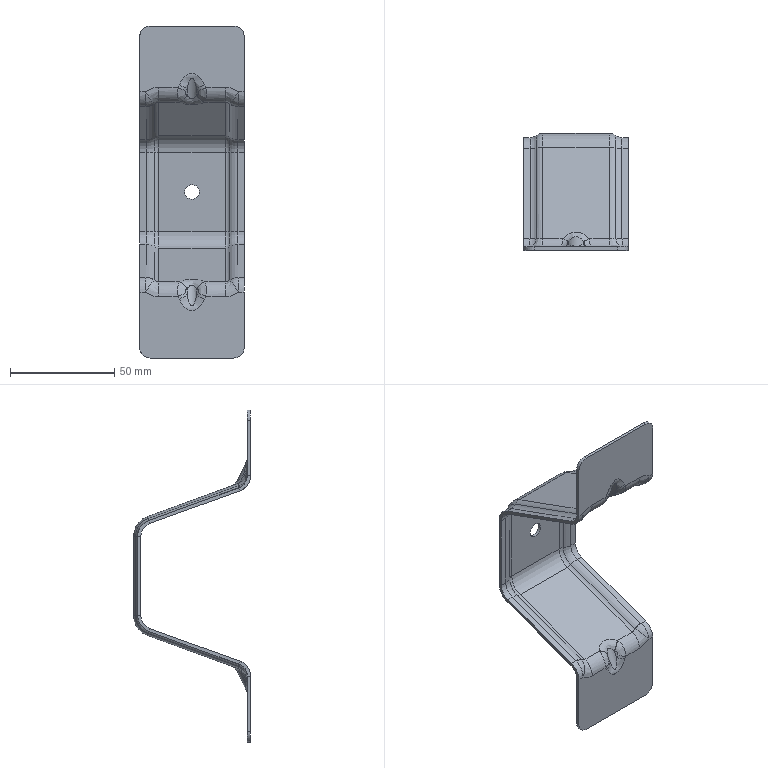Part | STEP file | FNA5401891 | 1 solid | 184 faces | box 50 x 55.964 x 158.896 mm | volume 17278 mm3 | cylinder 78 | spline 72 | plane 18 | torus 16 | commonest cylinder face diameters 10 x18 7 x10 13 x10 8 x8 11 x8 12 x8